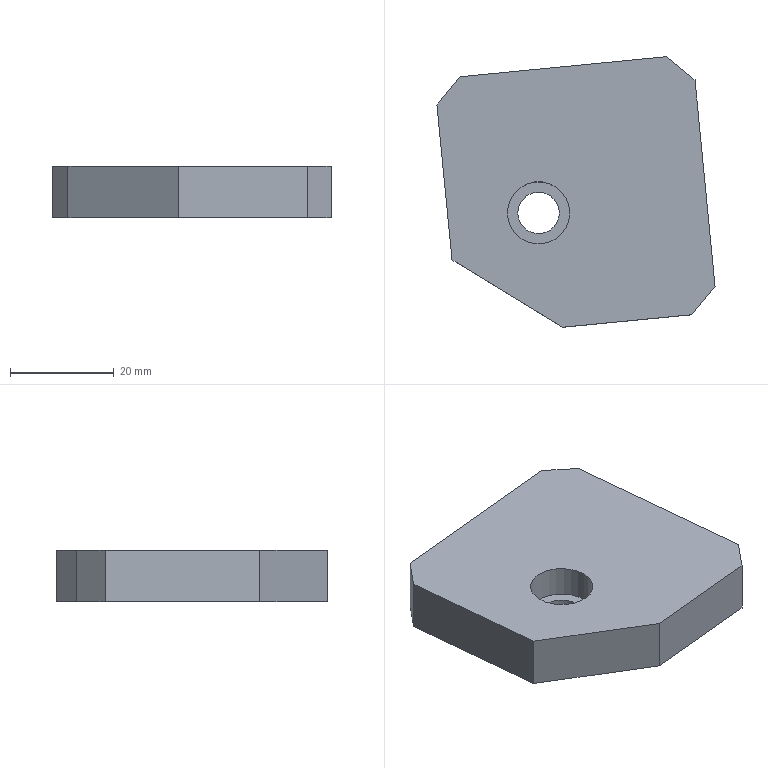Part | NX | features solid 2 | 1 solid | 13 faces | box 53.632 x 52.182 x 10 mm | volume 22245 mm3 | plane 11 | cylinder 2 | commonest cylinder face diameters 8 x1 12 x1
STEP:
#1=CARTESIAN_POINT('',(864.968,-152.567,148.));
#2=VERTEX_POINT('',#1);
#3=CARTESIAN_POINT('',(870.968,-152.567,148.));
#4=DIRECTION('',(0.,0.,1.));
#5=DIRECTION('',(-1.,0.,0.));
#6=AXIS2_PLACEMENT_3D('',#3,#4,#5);
#7=CIRCLE('',#6,6.);
#8=EDGE_CURVE('',#2,#2,#7,.F.);
#9=ORIENTED_EDGE('',*,*,#8,.T.);
#10=EDGE_LOOP('',(#9));
#11=FACE_BOUND('',#10,.T.);
#12=CARTESIAN_POINT('',(854.271,-161.627,148.));
#13=VERTEX_POINT('',#12);
#14=CARTESIAN_POINT('',(851.371,-131.767,148.));
#15=VERTEX_POINT('',#14);
#16=CARTESIAN_POINT('',(850.888,-126.79,148.));
#17=DIRECTION('',(-0.09666,0.9953,0.));
#18=VECTOR('',#17,1000.);
#19=LINE('',#16,#18);
#20=EDGE_CURVE('',#13,#15,#19,.T.);
#21=ORIENTED_EDGE('',*,*,#20,.F.);
#22=CARTESIAN_POINT('',(875.627,-174.623,148.));
#23=VERTEX_POINT('',#22);
#24=CARTESIAN_POINT('',(826.08,-144.471,148.));
#25=DIRECTION('',(0.8542,-0.5199,0.));
#26=VECTOR('',#25,1000.);
#27=LINE('',#24,#26);
#28=EDGE_CURVE('',#13,#23,#27,.T.);
#29=ORIENTED_EDGE('',*,*,#28,.T.);
#30=CARTESIAN_POINT('',(900.51,-172.207,148.));
#31=VERTEX_POINT('',#30);
#32=CARTESIAN_POINT('',(900.51,-172.207,148.));
#33=DIRECTION('',(-0.9953,-0.09666,0.));
#34=VECTOR('',#33,1000.);
#35=LINE('',#32,#34);
#36=EDGE_CURVE('',#31,#23,#35,.T.);
#37=ORIENTED_EDGE('',*,*,#36,.F.);
#38=CARTESIAN_POINT('',(905.003,-166.747,148.));
#39=VERTEX_POINT('',#38);
#40=CARTESIAN_POINT('',(896.016,-177.667,148.));
#41=DIRECTION('',(-0.6354,-0.7721,0.));
#42=VECTOR('',#41,1000.);
#43=LINE('',#40,#42);
#44=EDGE_CURVE('',#39,#31,#43,.T.);
#45=ORIENTED_EDGE('',*,*,#44,.F.);
#46=CARTESIAN_POINT('',(901.137,-126.934,148.));
#47=VERTEX_POINT('',#46);
#48=CARTESIAN_POINT('',(900.653,-121.957,148.));
#49=DIRECTION('',(-0.09666,0.9953,0.));
#50=VECTOR('',#49,1000.);
#51=LINE('',#48,#50);
#52=EDGE_CURVE('',#39,#47,#51,.T.);
#53=ORIENTED_EDGE('',*,*,#52,.T.);
#54=CARTESIAN_POINT('',(895.677,-122.441,148.));
#55=VERTEX_POINT('',#54);
#56=CARTESIAN_POINT('',(862.917,-95.481,148.));
#57=DIRECTION('',(0.7721,-0.6354,0.));
#58=VECTOR('',#57,1000.);
#59=LINE('',#56,#58);
#60=EDGE_CURVE('',#55,#47,#59,.T.);
#61=ORIENTED_EDGE('',*,*,#60,.F.);
#62=CARTESIAN_POINT('',(855.864,-126.307,148.));
#63=VERTEX_POINT('',#62);
#64=CARTESIAN_POINT('',(895.677,-122.441,148.));
#65=DIRECTION('',(-0.9953,-0.09666,0.));
#66=VECTOR('',#65,1000.);
#67=LINE('',#64,#66);
#68=EDGE_CURVE('',#55,#63,#67,.T.);
#69=ORIENTED_EDGE('',*,*,#68,.T.);
#70=CARTESIAN_POINT('',(855.864,-126.307,148.));
#71=DIRECTION('',(0.6354,0.7721,0.));
#72=VECTOR('',#71,1000.);
#73=LINE('',#70,#72);
#74=EDGE_CURVE('',#15,#63,#73,.T.);
#75=ORIENTED_EDGE('',*,*,#74,.F.);
#76=EDGE_LOOP('',(#21,#29,#37,#45,#53,#61,#69,#75));
#77=FACE_BOUND('',#76,.T.);
#78=CARTESIAN_POINT('',(835.958,-128.24,148.));
#79=DIRECTION('',(0.,0.,-1.));
#80=DIRECTION('',(-1.,0.,0.));
#81=AXIS2_PLACEMENT_3D('',#78,#79,#80);
#82=PLANE('',#81);
#83=ADVANCED_FACE('',(#11,#77),#82,.F.);
#84=CARTESIAN_POINT('',(866.968,-152.567,138.));
#85=VERTEX_POINT('',#84);
#86=CARTESIAN_POINT('',(870.968,-152.567,138.));
#87=DIRECTION('',(0.,0.,1.));
#88=DIRECTION('',(-1.,0.,0.));
#89=AXIS2_PLACEMENT_3D('',#86,#87,#88);
#90=CIRCLE('',#89,4.);
#91=EDGE_CURVE('',#85,#85,#90,.T.);
#92=ORIENTED_EDGE('',*,*,#91,.T.);
#93=EDGE_LOOP('',(#92));
#94=FACE_BOUND('',#93,.T.);
#95=CARTESIAN_POINT('',(895.677,-122.441,138.));
#96=VERTEX_POINT('',#95);
#97=CARTESIAN_POINT('',(855.864,-126.307,138.));
#98=VERTEX_POINT('',#97);
#99=CARTESIAN_POINT('',(895.677,-122.441,138.));
#100=DIRECTION('',(-0.9953,-0.09666,0.));
#101=VECTOR('',#100,1000.);
#102=LINE('',#99,#101);
#103=EDGE_CURVE('',#96,#98,#102,.T.);
#104=ORIENTED_EDGE('',*,*,#103,.F.);
#105=CARTESIAN_POINT('',(901.137,-126.934,138.));
#106=VERTEX_POINT('',#105);
#107=CARTESIAN_POINT('',(895.677,-122.441,138.));
#108=DIRECTION('',(0.7721,-0.6354,0.));
#109=VECTOR('',#108,1000.);
#110=LINE('',#107,#109);
#111=EDGE_CURVE('',#96,#106,#110,.T.);
#112=ORIENTED_EDGE('',*,*,#111,.T.);
#113=CARTESIAN_POINT('',(905.003,-166.747,138.));
#114=VERTEX_POINT('',#113);
#115=CARTESIAN_POINT('',(900.653,-121.957,138.));
#116=DIRECTION('',(-0.09666,0.9953,0.));
#117=VECTOR('',#116,1000.);
#118=LINE('',#115,#117);
#119=EDGE_CURVE('',#114,#106,#118,.T.);
#120=ORIENTED_EDGE('',*,*,#119,.F.);
#121=CARTESIAN_POINT('',(900.51,-172.207,138.));
#122=VERTEX_POINT('',#121);
#123=CARTESIAN_POINT('',(905.003,-166.747,138.));
#124=DIRECTION('',(-0.6354,-0.7721,0.));
#125=VECTOR('',#124,1000.);
#126=LINE('',#123,#125);
#127=EDGE_CURVE('',#114,#122,#126,.T.);
#128=ORIENTED_EDGE('',*,*,#127,.T.);
#129=CARTESIAN_POINT('',(875.627,-174.623,138.));
#130=VERTEX_POINT('',#129);
#131=CARTESIAN_POINT('',(900.51,-172.207,138.));
#132=DIRECTION('',(-0.9953,-0.09666,0.));
#133=VECTOR('',#132,1000.);
#134=LINE('',#131,#133);
#135=EDGE_CURVE('',#122,#130,#134,.T.);
#136=ORIENTED_EDGE('',*,*,#135,.T.);
#137=CARTESIAN_POINT('',(854.271,-161.627,138.));
#138=VERTEX_POINT('',#137);
#139=CARTESIAN_POINT('',(854.271,-161.627,138.));
#140=DIRECTION('',(0.8542,-0.5199,0.));
#141=VECTOR('',#140,1000.);
#142=LINE('',#139,#141);
#143=EDGE_CURVE('',#138,#130,#142,.T.);
#144=ORIENTED_EDGE('',*,*,#143,.F.);
#145=CARTESIAN_POINT('',(851.371,-131.767,138.));
#146=VERTEX_POINT('',#145);
#147=CARTESIAN_POINT('',(855.72,-176.556,138.));
#148=DIRECTION('',(0.09666,-0.9953,0.));
#149=VECTOR('',#148,1000.);
#150=LINE('',#147,#149);
#151=EDGE_CURVE('',#146,#138,#150,.T.);
#152=ORIENTED_EDGE('',*,*,#151,.F.);
#153=CARTESIAN_POINT('',(846.878,-137.227,138.));
#154=DIRECTION('',(-0.6354,-0.7721,0.));
#155=VECTOR('',#154,1000.);
#156=LINE('',#153,#155);
#157=EDGE_CURVE('',#98,#146,#156,.T.);
#158=ORIENTED_EDGE('',*,*,#157,.F.);
#159=EDGE_LOOP('',(#104,#112,#120,#128,#136,#144,#152,#158));
#160=FACE_BOUND('',#159,.T.);
#161=CARTESIAN_POINT('',(835.958,-128.24,138.));
#162=DIRECTION('',(0.,0.,-1.));
#163=DIRECTION('',(-1.,0.,0.));
#164=AXIS2_PLACEMENT_3D('',#161,#162,#163);
#165=PLANE('',#164);
#166=ADVANCED_FACE('',(#94,#160),#165,.T.);
#167=CARTESIAN_POINT('',(875.627,-174.623,338.));
#168=DIRECTION('',(0.,0.,-1.));
#169=VECTOR('',#168,1000.);
#170=LINE('',#167,#169);
#171=EDGE_CURVE('',#23,#130,#170,.T.);
#172=ORIENTED_EDGE('',*,*,#171,.T.);
#173=ORIENTED_EDGE('',*,*,#135,.F.);
#174=CARTESIAN_POINT('',(900.51,-172.207,168.));
#175=DIRECTION('',(0.,0.,-1.));
#176=VECTOR('',#175,1000.);
#177=LINE('',#174,#176);
#178=EDGE_CURVE('',#31,#122,#177,.T.);
#179=ORIENTED_EDGE('',*,*,#178,.F.);
#180=ORIENTED_EDGE('',*,*,#36,.T.);
#181=EDGE_LOOP('',(#172,#173,#179,#180));
#182=FACE_BOUND('',#181,.T.);
#183=CARTESIAN_POINT('',(900.51,-172.207,148.));
#184=DIRECTION('',(-0.09666,0.9953,0.));
#185=DIRECTION('',(0.9953,0.09666,0.));
#186=AXIS2_PLACEMENT_3D('',#183,#184,#185);
#187=PLANE('',#186);
#188=ADVANCED_FACE('',(#182),#187,.F.);
#189=ORIENTED_EDGE('',*,*,#151,.T.);
#190=CARTESIAN_POINT('',(854.271,-161.627,338.));
#191=DIRECTION('',(0.,0.,-1.));
#192=VECTOR('',#191,1000.);
#193=LINE('',#190,#192);
#194=EDGE_CURVE('',#13,#138,#193,.T.);
#195=ORIENTED_EDGE('',*,*,#194,.F.);
#196=ORIENTED_EDGE('',*,*,#20,.T.);
#197=CARTESIAN_POINT('',(851.371,-131.767,148.));
#198=DIRECTION('',(0.,0.,1.));
#199=VECTOR('',#198,1000.);
#200=LINE('',#197,#199);
#201=EDGE_CURVE('',#146,#15,#200,.T.);
#202=ORIENTED_EDGE('',*,*,#201,.F.);
#203=EDGE_LOOP('',(#189,#195,#196,#202));
#204=FACE_BOUND('',#203,.T.);
#205=CARTESIAN_POINT('',(855.72,-176.556,148.));
#206=DIRECTION('',(0.9953,0.09666,0.));
#207=DIRECTION('',(0.09666,-0.9953,0.));
#208=AXIS2_PLACEMENT_3D('',#205,#206,#207);
#209=PLANE('',#208);
#210=ADVANCED_FACE('',(#204),#209,.F.);
#211=CARTESIAN_POINT('',(905.003,-166.747,168.));
#212=DIRECTION('',(0.,0.,-1.));
#213=VECTOR('',#212,1000.);
#214=LINE('',#211,#213);
#215=EDGE_CURVE('',#39,#114,#214,.T.);
#216=ORIENTED_EDGE('',*,*,#215,.T.);
#217=ORIENTED_EDGE('',*,*,#119,.T.);
#218=CARTESIAN_POINT('',(901.137,-126.934,168.));
#219=DIRECTION('',(0.,0.,-1.));
#220=VECTOR('',#219,1000.);
#221=LINE('',#218,#220);
#222=EDGE_CURVE('',#47,#106,#221,.T.);
#223=ORIENTED_EDGE('',*,*,#222,.F.);
#224=ORIENTED_EDGE('',*,*,#52,.F.);
#225=EDGE_LOOP('',(#216,#217,#223,#224));
#226=FACE_BOUND('',#225,.T.);
#227=CARTESIAN_POINT('',(905.486,-171.723,148.));
#228=DIRECTION('',(0.9953,0.09666,0.));
#229=DIRECTION('',(0.09666,-0.9953,0.));
#230=AXIS2_PLACEMENT_3D('',#227,#228,#229);
#231=PLANE('',#230);
#232=ADVANCED_FACE('',(#226),#231,.T.);
#233=ORIENTED_EDGE('',*,*,#68,.F.);
#234=CARTESIAN_POINT('',(895.677,-122.441,168.));
#235=DIRECTION('',(0.,0.,-1.));
#236=VECTOR('',#235,1000.);
#237=LINE('',#234,#236);
#238=EDGE_CURVE('',#55,#96,#237,.T.);
#239=ORIENTED_EDGE('',*,*,#238,.T.);
#240=ORIENTED_EDGE('',*,*,#103,.T.);
#241=CARTESIAN_POINT('',(855.864,-126.307,138.));
#242=DIRECTION('',(0.,0.,-1.));
#243=VECTOR('',#242,1000.);
#244=LINE('',#241,#243);
#245=EDGE_CURVE('',#63,#98,#244,.T.);
#246=ORIENTED_EDGE('',*,*,#245,.F.);
#247=EDGE_LOOP('',(#233,#239,#240,#246));
#248=FACE_BOUND('',#247,.T.);
#249=CARTESIAN_POINT('',(895.677,-122.441,148.));
#250=DIRECTION('',(-0.09666,0.9953,0.));
#251=DIRECTION('',(0.9953,0.09666,0.));
#252=AXIS2_PLACEMENT_3D('',#249,#250,#251);
#253=PLANE('',#252);
#254=ADVANCED_FACE('',(#248),#253,.T.);
#255=CARTESIAN_POINT('',(876.968,-152.567,142.));
#256=VERTEX_POINT('',#255);
#257=CARTESIAN_POINT('',(870.968,-152.567,142.));
#258=DIRECTION('',(0.,0.,-1.));
#259=DIRECTION('',(1.,0.,0.));
#260=AXIS2_PLACEMENT_3D('',#257,#258,#259);
#261=CIRCLE('',#260,6.);
#262=EDGE_CURVE('',#256,#256,#261,.T.);
#263=ORIENTED_EDGE('',*,*,#262,.T.);
#264=EDGE_LOOP('',(#263));
#265=FACE_BOUND('',#264,.T.);
#266=ORIENTED_EDGE('',*,*,#8,.F.);
#267=EDGE_LOOP('',(#266));
#268=FACE_BOUND('',#267,.T.);
#269=CARTESIAN_POINT('',(870.968,-152.567,162.));
#270=DIRECTION('',(0.,0.,-1.));
#271=DIRECTION('',(-1.,0.,0.));
#272=AXIS2_PLACEMENT_3D('',#269,#270,#271);
#273=CYLINDRICAL_SURFACE('',#272,6.);
#274=ADVANCED_FACE('',(#265,#268),#273,.F.);
#275=ORIENTED_EDGE('',*,*,#262,.F.);
#276=EDGE_LOOP('',(#275));
#277=FACE_BOUND('',#276,.T.);
#278=CARTESIAN_POINT('',(874.968,-152.567,142.));
#279=VERTEX_POINT('',#278);
#280=CARTESIAN_POINT('',(870.968,-152.567,142.));
#281=DIRECTION('',(0.,0.,-1.));
#282=DIRECTION('',(1.,0.,0.));
#283=AXIS2_PLACEMENT_3D('',#280,#281,#282);
#284=CIRCLE('',#283,4.);
#285=EDGE_CURVE('',#279,#279,#284,.F.);
#286=ORIENTED_EDGE('',*,*,#285,.F.);
#287=EDGE_LOOP('',(#286));
#288=FACE_BOUND('',#287,.T.);
#289=CARTESIAN_POINT('',(870.968,-152.567,142.));
#290=DIRECTION('',(0.,0.,1.));
#291=DIRECTION('',(1.,0.,0.));
#292=AXIS2_PLACEMENT_3D('',#289,#290,#291);
#293=PLANE('',#292);
#294=ADVANCED_FACE('',(#277,#288),#293,.T.);
#295=ORIENTED_EDGE('',*,*,#91,.F.);
#296=EDGE_LOOP('',(#295));
#297=FACE_BOUND('',#296,.T.);
#298=ORIENTED_EDGE('',*,*,#285,.T.);
#299=EDGE_LOOP('',(#298));
#300=FACE_BOUND('',#299,.T.);
#301=CARTESIAN_POINT('',(870.968,-152.567,162.));
#302=DIRECTION('',(0.,0.,-1.));
#303=DIRECTION('',(-0.09666,0.9953,0.));
#304=AXIS2_PLACEMENT_3D('',#301,#302,#303);
#305=CYLINDRICAL_SURFACE('',#304,4.);
#306=ADVANCED_FACE('',(#297,#300),#305,.F.);
#307=ORIENTED_EDGE('',*,*,#238,.F.);
#308=ORIENTED_EDGE('',*,*,#60,.T.);
#309=ORIENTED_EDGE('',*,*,#222,.T.);
#310=ORIENTED_EDGE('',*,*,#111,.F.);
#311=EDGE_LOOP('',(#307,#308,#309,#310));
#312=FACE_BOUND('',#311,.T.);
#313=CARTESIAN_POINT('',(895.677,-122.441,168.));
#314=DIRECTION('',(-0.6354,-0.7721,0.));
#315=DIRECTION('',(-0.7721,0.6354,0.));
#316=AXIS2_PLACEMENT_3D('',#313,#314,#315);
#317=PLANE('',#316);
#318=ADVANCED_FACE('',(#312),#317,.F.);
#319=ORIENTED_EDGE('',*,*,#215,.F.);
#320=ORIENTED_EDGE('',*,*,#44,.T.);
#321=ORIENTED_EDGE('',*,*,#178,.T.);
#322=ORIENTED_EDGE('',*,*,#127,.F.);
#323=EDGE_LOOP('',(#319,#320,#321,#322));
#324=FACE_BOUND('',#323,.T.);
#325=CARTESIAN_POINT('',(905.003,-166.747,168.));
#326=DIRECTION('',(-0.7721,0.6354,0.));
#327=DIRECTION('',(0.6354,0.7721,0.));
#328=AXIS2_PLACEMENT_3D('',#325,#326,#327);
#329=PLANE('',#328);
#330=ADVANCED_FACE('',(#324),#329,.F.);
#331=ORIENTED_EDGE('',*,*,#28,.F.);
#332=ORIENTED_EDGE('',*,*,#194,.T.);
#333=ORIENTED_EDGE('',*,*,#143,.T.);
#334=ORIENTED_EDGE('',*,*,#171,.F.);
#335=EDGE_LOOP('',(#331,#332,#333,#334));
#336=FACE_BOUND('',#335,.T.);
#337=CARTESIAN_POINT('',(854.271,-161.627,338.));
#338=DIRECTION('',(-0.5199,-0.8542,0.));
#339=DIRECTION('',(-0.8542,0.5199,0.));
#340=AXIS2_PLACEMENT_3D('',#337,#338,#339);
#341=PLANE('',#340);
#342=ADVANCED_FACE('',(#336),#341,.T.);
#343=ORIENTED_EDGE('',*,*,#74,.T.);
#344=ORIENTED_EDGE('',*,*,#245,.T.);
#345=ORIENTED_EDGE('',*,*,#157,.T.);
#346=ORIENTED_EDGE('',*,*,#201,.T.);
#347=EDGE_LOOP('',(#343,#344,#345,#346));
#348=FACE_BOUND('',#347,.T.);
#349=CARTESIAN_POINT('',(855.864,-126.307,148.));
#350=DIRECTION('',(-0.7721,0.6354,0.));
#351=DIRECTION('',(0.6354,0.7721,0.));
#352=AXIS2_PLACEMENT_3D('',#349,#350,#351);
#353=PLANE('',#352);
#354=ADVANCED_FACE('',(#348),#353,.T.);
#355=CLOSED_SHELL('',(#83,#166,#188,#210,#232,#254,#274,#294,#306,#318,#330,#342,#354));
#356=MANIFOLD_SOLID_BREP('',#355);
#357=(LENGTH_UNIT()NAMED_UNIT(*)SI_UNIT(.MILLI.,.METRE.));
#358=UNCERTAINTY_MEASURE_WITH_UNIT(LENGTH_MEASURE(0.00001),#357,'','');
#359=(NAMED_UNIT(*)PLANE_ANGLE_UNIT()SI_UNIT($,.RADIAN.));
#360=(NAMED_UNIT(*)SI_UNIT($,.STERADIAN.)SOLID_ANGLE_UNIT());
#361=(GEOMETRIC_REPRESENTATION_CONTEXT(3)GLOBAL_UNCERTAINTY_ASSIGNED_CONTEXT((#358))GLOBAL_UNIT_ASSIGNED_CONTEXT((#357,#359,#360))REPRESENTATION_CONTEXT('',''));
#362=ADVANCED_BREP_SHAPE_REPRESENTATION('',(#356),#361);